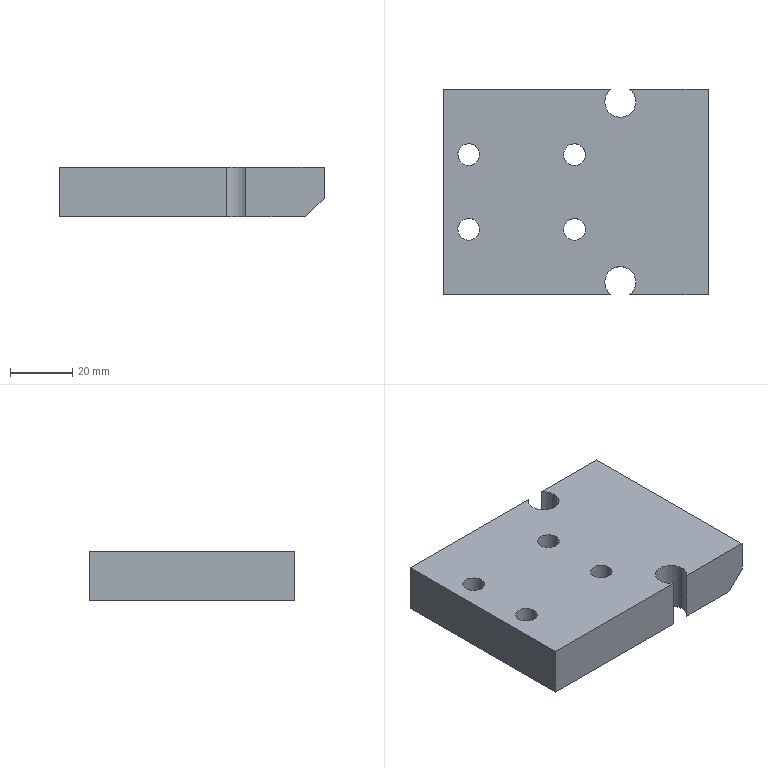Part | STEP file | Positioning_id2086_x_t | 1 solid | 19 faces | box 85 x 66 x 16 mm | volume 83727 mm3 | cylinder 10 | plane 9 | commonest cylinder face diameters 7 x8 10 x2